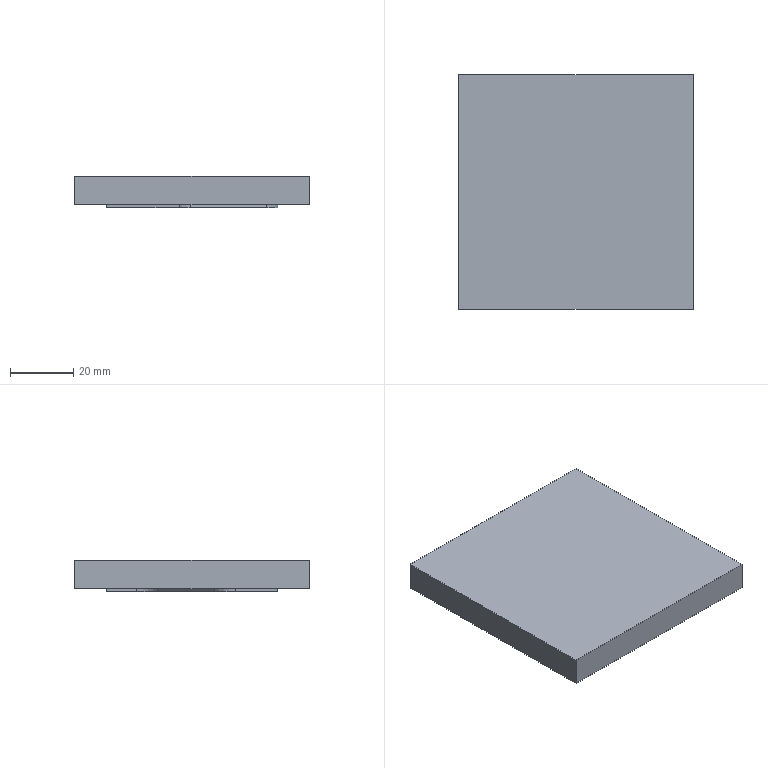Part | 2 solids | 58 faces | box 74 x 74 x 10 mm | volume 50306 mm3 | plane 35 | cylinder 23 | commonest cylinder face diameters 3 x12 16 x8 2.5 x2 2 x1